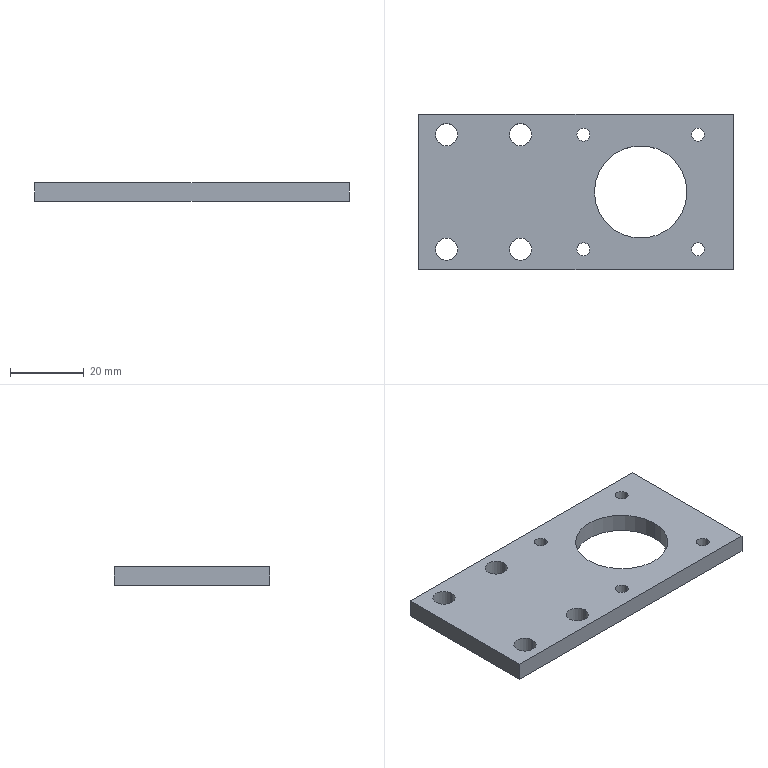Part | STEP file | Lead screw motor drive mounting plate split V1.201001 | 1 solid | 24 faces | box 85 x 42 x 5 mm | volume 14638 mm3 | cylinder 18 | plane 6 | commonest cylinder face diameters 3.5 x8 6 x8 25 x2